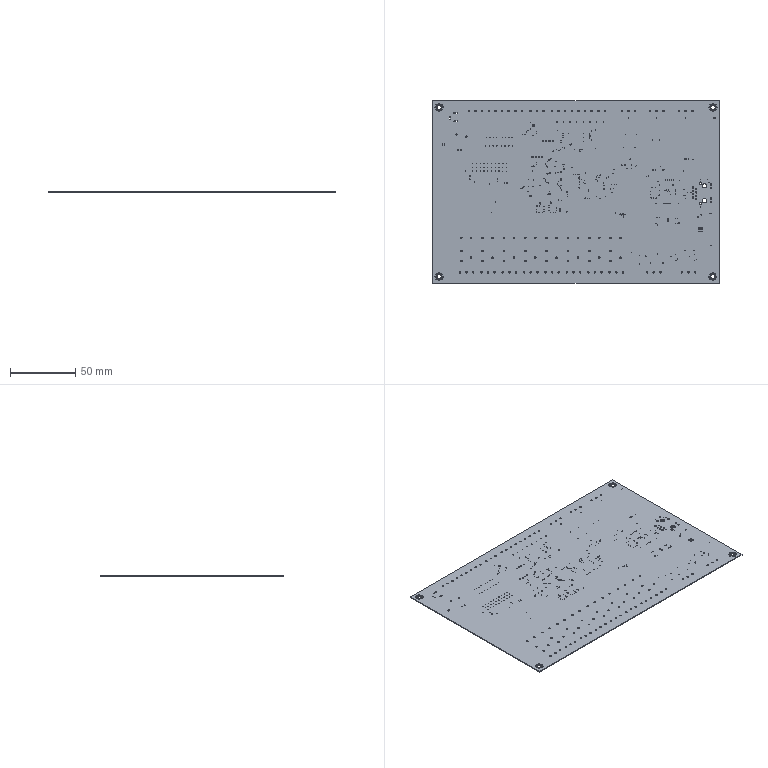Part | NX | features BREP 1 | 1 solid | 1082 faces | box 219.975 x 139.975 x 0.6237 mm | volume 19052 mm3 | cylinder 1070 | plane 12 | commonest cylinder face diameters 0.305 x732 1.2 x200 1 x100 0.8 x14 1.1 x8 3.2 x8